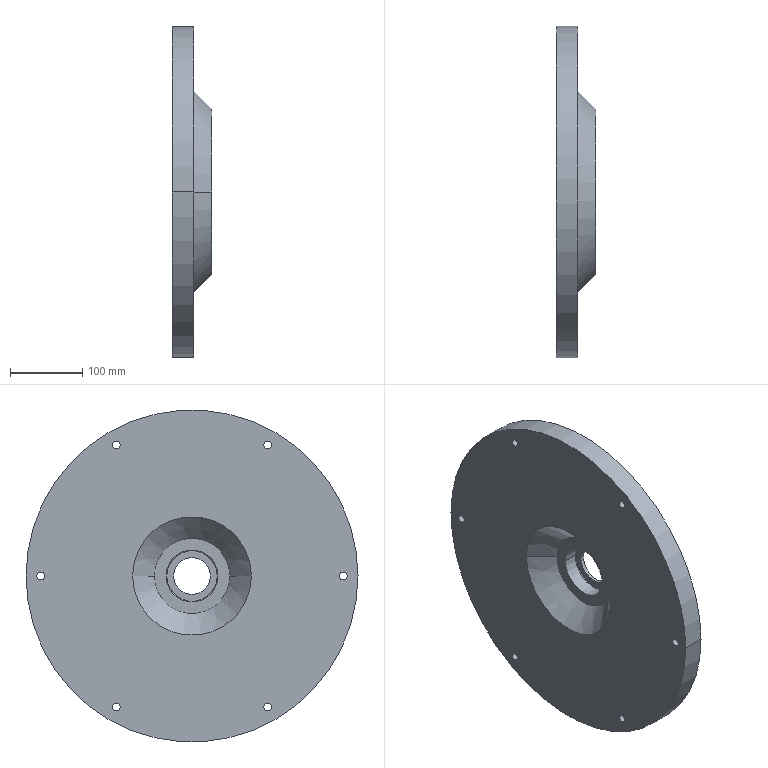Part | SolidWorks | features Cut 1, Revolution 1 | 1 solid | 29 faces | box 55 x 461 x 461 mm | volume 5743075 mm3 | cylinder 18 | plane 5 | cone 4 | torus 2 | commonest cylinder face diameters 11 x12 51 x2 72 x2 461 x2
STEP:
#1=CARTESIAN_POINT('',(-25.,204.5,0.));
#2=VERTEX_POINT('',#1);
#3=CARTESIAN_POINT('',(-25.,215.5,0.));
#4=VERTEX_POINT('',#3);
#5=CARTESIAN_POINT('',(-25.,210.,0.));
#6=DIRECTION('',(1.,0.,0.));
#7=DIRECTION('',(0.,1.,0.));
#8=AXIS2_PLACEMENT_3D('',#5,#6,#7);
#9=CIRCLE('',#8,5.5);
#10=EDGE_CURVE('',#2,#4,#9,.T.);
#11=ORIENTED_EDGE('',*,*,#10,.T.);
#12=CARTESIAN_POINT('',(-55.,215.5,0.));
#13=VERTEX_POINT('',#12);
#14=CARTESIAN_POINT('',(30.,215.5,0.));
#15=DIRECTION('',(-1.,0.,0.));
#16=VECTOR('',#15,1000.);
#17=LINE('',#14,#16);
#18=EDGE_CURVE('',#4,#13,#17,.T.);
#19=ORIENTED_EDGE('',*,*,#18,.T.);
#20=CARTESIAN_POINT('',(-55.,204.5,0.));
#21=VERTEX_POINT('',#20);
#22=CARTESIAN_POINT('',(-55.,210.,0.));
#23=DIRECTION('',(-1.,0.,0.));
#24=DIRECTION('',(0.,-1.,0.));
#25=AXIS2_PLACEMENT_3D('',#22,#23,#24);
#26=CIRCLE('',#25,5.5);
#27=EDGE_CURVE('',#13,#21,#26,.T.);
#28=ORIENTED_EDGE('',*,*,#27,.T.);
#29=CARTESIAN_POINT('',(30.,204.5,0.));
#30=DIRECTION('',(-1.,0.,0.));
#31=VECTOR('',#30,1000.);
#32=LINE('',#29,#31);
#33=EDGE_CURVE('',#2,#21,#32,.T.);
#34=ORIENTED_EDGE('',*,*,#33,.F.);
#35=EDGE_LOOP('',(#11,#19,#28,#34));
#36=FACE_OUTER_BOUND('',#35,.T.);
#37=CARTESIAN_POINT('',(30.,210.,0.));
#38=DIRECTION('',(-1.,0.,0.));
#39=DIRECTION('',(0.,-1.,0.));
#40=AXIS2_PLACEMENT_3D('',#37,#38,#39);
#41=CYLINDRICAL_SURFACE('',#40,5.5);
#42=ADVANCED_FACE('',(#36),#41,.F.);
#43=CARTESIAN_POINT('',(-25.,99.5,-181.865));
#44=VERTEX_POINT('',#43);
#45=CARTESIAN_POINT('',(-25.,110.5,-181.865));
#46=VERTEX_POINT('',#45);
#47=CARTESIAN_POINT('',(-25.,105.,-181.865));
#48=DIRECTION('',(1.,0.,0.));
#49=DIRECTION('',(0.,1.,0.));
#50=AXIS2_PLACEMENT_3D('',#47,#48,#49);
#51=CIRCLE('',#50,5.5);
#52=EDGE_CURVE('',#44,#46,#51,.T.);
#53=ORIENTED_EDGE('',*,*,#52,.T.);
#54=CARTESIAN_POINT('',(-55.,110.5,-181.865));
#55=VERTEX_POINT('',#54);
#56=CARTESIAN_POINT('',(30.,110.5,-181.865));
#57=DIRECTION('',(-1.,0.,0.));
#58=VECTOR('',#57,1000.);
#59=LINE('',#56,#58);
#60=EDGE_CURVE('',#46,#55,#59,.T.);
#61=ORIENTED_EDGE('',*,*,#60,.T.);
#62=CARTESIAN_POINT('',(-55.,99.5,-181.865));
#63=VERTEX_POINT('',#62);
#64=CARTESIAN_POINT('',(-55.,105.,-181.865));
#65=DIRECTION('',(-1.,0.,0.));
#66=DIRECTION('',(0.,-1.,0.));
#67=AXIS2_PLACEMENT_3D('',#64,#65,#66);
#68=CIRCLE('',#67,5.5);
#69=EDGE_CURVE('',#55,#63,#68,.T.);
#70=ORIENTED_EDGE('',*,*,#69,.T.);
#71=CARTESIAN_POINT('',(30.,99.5,-181.865));
#72=DIRECTION('',(-1.,0.,0.));
#73=VECTOR('',#72,1000.);
#74=LINE('',#71,#73);
#75=EDGE_CURVE('',#44,#63,#74,.T.);
#76=ORIENTED_EDGE('',*,*,#75,.F.);
#77=EDGE_LOOP('',(#53,#61,#70,#76));
#78=FACE_OUTER_BOUND('',#77,.T.);
#79=CARTESIAN_POINT('',(30.,105.,-181.865));
#80=DIRECTION('',(-1.,0.,0.));
#81=DIRECTION('',(0.,-1.,0.));
#82=AXIS2_PLACEMENT_3D('',#79,#80,#81);
#83=CYLINDRICAL_SURFACE('',#82,5.5);
#84=ADVANCED_FACE('',(#78),#83,.F.);
#85=CARTESIAN_POINT('',(-25.,-110.5,-181.865));
#86=VERTEX_POINT('',#85);
#87=CARTESIAN_POINT('',(-25.,-99.5,-181.865));
#88=VERTEX_POINT('',#87);
#89=CARTESIAN_POINT('',(-25.,-105.,-181.865));
#90=DIRECTION('',(1.,0.,0.));
#91=DIRECTION('',(0.,1.,0.));
#92=AXIS2_PLACEMENT_3D('',#89,#90,#91);
#93=CIRCLE('',#92,5.5);
#94=EDGE_CURVE('',#86,#88,#93,.T.);
#95=ORIENTED_EDGE('',*,*,#94,.T.);
#96=CARTESIAN_POINT('',(-55.,-99.5,-181.865));
#97=VERTEX_POINT('',#96);
#98=CARTESIAN_POINT('',(30.,-99.5,-181.865));
#99=DIRECTION('',(-1.,0.,0.));
#100=VECTOR('',#99,1000.);
#101=LINE('',#98,#100);
#102=EDGE_CURVE('',#88,#97,#101,.T.);
#103=ORIENTED_EDGE('',*,*,#102,.T.);
#104=CARTESIAN_POINT('',(-55.,-110.5,-181.865));
#105=VERTEX_POINT('',#104);
#106=CARTESIAN_POINT('',(-55.,-105.,-181.865));
#107=DIRECTION('',(-1.,0.,0.));
#108=DIRECTION('',(0.,-1.,0.));
#109=AXIS2_PLACEMENT_3D('',#106,#107,#108);
#110=CIRCLE('',#109,5.5);
#111=EDGE_CURVE('',#97,#105,#110,.T.);
#112=ORIENTED_EDGE('',*,*,#111,.T.);
#113=CARTESIAN_POINT('',(30.,-110.5,-181.865));
#114=DIRECTION('',(-1.,0.,0.));
#115=VECTOR('',#114,1000.);
#116=LINE('',#113,#115);
#117=EDGE_CURVE('',#86,#105,#116,.T.);
#118=ORIENTED_EDGE('',*,*,#117,.F.);
#119=EDGE_LOOP('',(#95,#103,#112,#118));
#120=FACE_OUTER_BOUND('',#119,.T.);
#121=CARTESIAN_POINT('',(30.,-105.,-181.865));
#122=DIRECTION('',(-1.,0.,0.));
#123=DIRECTION('',(0.,-1.,0.));
#124=AXIS2_PLACEMENT_3D('',#121,#122,#123);
#125=CYLINDRICAL_SURFACE('',#124,5.5);
#126=ADVANCED_FACE('',(#120),#125,.F.);
#127=CARTESIAN_POINT('',(-25.,-215.5,0.));
#128=VERTEX_POINT('',#127);
#129=CARTESIAN_POINT('',(-25.,-204.5,0.));
#130=VERTEX_POINT('',#129);
#131=CARTESIAN_POINT('',(-25.,-210.,0.));
#132=DIRECTION('',(1.,0.,0.));
#133=DIRECTION('',(0.,1.,0.));
#134=AXIS2_PLACEMENT_3D('',#131,#132,#133);
#135=CIRCLE('',#134,5.5);
#136=EDGE_CURVE('',#128,#130,#135,.T.);
#137=ORIENTED_EDGE('',*,*,#136,.T.);
#138=CARTESIAN_POINT('',(-55.,-204.5,0.));
#139=VERTEX_POINT('',#138);
#140=CARTESIAN_POINT('',(30.,-204.5,0.));
#141=DIRECTION('',(-1.,0.,0.));
#142=VECTOR('',#141,1000.);
#143=LINE('',#140,#142);
#144=EDGE_CURVE('',#130,#139,#143,.T.);
#145=ORIENTED_EDGE('',*,*,#144,.T.);
#146=CARTESIAN_POINT('',(-55.,-215.5,0.));
#147=VERTEX_POINT('',#146);
#148=CARTESIAN_POINT('',(-55.,-210.,0.));
#149=DIRECTION('',(-1.,0.,0.));
#150=DIRECTION('',(0.,-1.,0.));
#151=AXIS2_PLACEMENT_3D('',#148,#149,#150);
#152=CIRCLE('',#151,5.5);
#153=EDGE_CURVE('',#139,#147,#152,.T.);
#154=ORIENTED_EDGE('',*,*,#153,.T.);
#155=CARTESIAN_POINT('',(30.,-215.5,0.));
#156=DIRECTION('',(-1.,0.,0.));
#157=VECTOR('',#156,1000.);
#158=LINE('',#155,#157);
#159=EDGE_CURVE('',#128,#147,#158,.T.);
#160=ORIENTED_EDGE('',*,*,#159,.F.);
#161=EDGE_LOOP('',(#137,#145,#154,#160));
#162=FACE_OUTER_BOUND('',#161,.T.);
#163=CARTESIAN_POINT('',(30.,-210.,0.));
#164=DIRECTION('',(-1.,0.,0.));
#165=DIRECTION('',(0.,-1.,0.));
#166=AXIS2_PLACEMENT_3D('',#163,#164,#165);
#167=CYLINDRICAL_SURFACE('',#166,5.5);
#168=ADVANCED_FACE('',(#162),#167,.F.);
#169=CARTESIAN_POINT('',(-25.,-110.5,181.865));
#170=VERTEX_POINT('',#169);
#171=CARTESIAN_POINT('',(-25.,-99.5,181.865));
#172=VERTEX_POINT('',#171);
#173=CARTESIAN_POINT('',(-25.,-105.,181.865));
#174=DIRECTION('',(1.,0.,0.));
#175=DIRECTION('',(0.,1.,0.));
#176=AXIS2_PLACEMENT_3D('',#173,#174,#175);
#177=CIRCLE('',#176,5.5);
#178=EDGE_CURVE('',#170,#172,#177,.T.);
#179=ORIENTED_EDGE('',*,*,#178,.T.);
#180=CARTESIAN_POINT('',(-55.,-99.5,181.865));
#181=VERTEX_POINT('',#180);
#182=CARTESIAN_POINT('',(30.,-99.5,181.865));
#183=DIRECTION('',(-1.,0.,0.));
#184=VECTOR('',#183,1000.);
#185=LINE('',#182,#184);
#186=EDGE_CURVE('',#172,#181,#185,.T.);
#187=ORIENTED_EDGE('',*,*,#186,.T.);
#188=CARTESIAN_POINT('',(-55.,-110.5,181.865));
#189=VERTEX_POINT('',#188);
#190=CARTESIAN_POINT('',(-55.,-105.,181.865));
#191=DIRECTION('',(-1.,0.,0.));
#192=DIRECTION('',(0.,-1.,0.));
#193=AXIS2_PLACEMENT_3D('',#190,#191,#192);
#194=CIRCLE('',#193,5.5);
#195=EDGE_CURVE('',#181,#189,#194,.T.);
#196=ORIENTED_EDGE('',*,*,#195,.T.);
#197=CARTESIAN_POINT('',(30.,-110.5,181.865));
#198=DIRECTION('',(-1.,0.,0.));
#199=VECTOR('',#198,1000.);
#200=LINE('',#197,#199);
#201=EDGE_CURVE('',#170,#189,#200,.T.);
#202=ORIENTED_EDGE('',*,*,#201,.F.);
#203=EDGE_LOOP('',(#179,#187,#196,#202));
#204=FACE_OUTER_BOUND('',#203,.T.);
#205=CARTESIAN_POINT('',(30.,-105.,181.865));
#206=DIRECTION('',(-1.,0.,0.));
#207=DIRECTION('',(0.,-1.,0.));
#208=AXIS2_PLACEMENT_3D('',#205,#206,#207);
#209=CYLINDRICAL_SURFACE('',#208,5.5);
#210=ADVANCED_FACE('',(#204),#209,.F.);
#211=CARTESIAN_POINT('',(-25.,99.5,181.865));
#212=VERTEX_POINT('',#211);
#213=CARTESIAN_POINT('',(-25.,110.5,181.865));
#214=VERTEX_POINT('',#213);
#215=CARTESIAN_POINT('',(-25.,105.,181.865));
#216=DIRECTION('',(1.,0.,0.));
#217=DIRECTION('',(0.,1.,0.));
#218=AXIS2_PLACEMENT_3D('',#215,#216,#217);
#219=CIRCLE('',#218,5.5);
#220=EDGE_CURVE('',#212,#214,#219,.T.);
#221=ORIENTED_EDGE('',*,*,#220,.T.);
#222=CARTESIAN_POINT('',(-55.,110.5,181.865));
#223=VERTEX_POINT('',#222);
#224=CARTESIAN_POINT('',(30.,110.5,181.865));
#225=DIRECTION('',(-1.,0.,0.));
#226=VECTOR('',#225,1000.);
#227=LINE('',#224,#226);
#228=EDGE_CURVE('',#214,#223,#227,.T.);
#229=ORIENTED_EDGE('',*,*,#228,.T.);
#230=CARTESIAN_POINT('',(-55.,99.5,181.865));
#231=VERTEX_POINT('',#230);
#232=CARTESIAN_POINT('',(-55.,105.,181.865));
#233=DIRECTION('',(-1.,0.,0.));
#234=DIRECTION('',(0.,-1.,0.));
#235=AXIS2_PLACEMENT_3D('',#232,#233,#234);
#236=CIRCLE('',#235,5.5);
#237=EDGE_CURVE('',#223,#231,#236,.T.);
#238=ORIENTED_EDGE('',*,*,#237,.T.);
#239=CARTESIAN_POINT('',(30.,99.5,181.865));
#240=DIRECTION('',(-1.,0.,0.));
#241=VECTOR('',#240,1000.);
#242=LINE('',#239,#241);
#243=EDGE_CURVE('',#212,#231,#242,.T.);
#244=ORIENTED_EDGE('',*,*,#243,.F.);
#245=EDGE_LOOP('',(#221,#229,#238,#244));
#246=FACE_OUTER_BOUND('',#245,.T.);
#247=CARTESIAN_POINT('',(30.,105.,181.865));
#248=DIRECTION('',(-1.,0.,0.));
#249=DIRECTION('',(0.,-1.,0.));
#250=AXIS2_PLACEMENT_3D('',#247,#248,#249);
#251=CYLINDRICAL_SURFACE('',#250,5.5);
#252=ADVANCED_FACE('',(#246),#251,.F.);
#253=CARTESIAN_POINT('',(0.,115.,0.));
#254=VERTEX_POINT('',#253);
#255=CARTESIAN_POINT('',(0.,-115.,0.));
#256=VERTEX_POINT('',#255);
#257=CARTESIAN_POINT('',(0.,0.,0.));
#258=DIRECTION('',(1.,0.,0.));
#259=DIRECTION('',(0.,1.,0.));
#260=AXIS2_PLACEMENT_3D('',#257,#258,#259);
#261=CIRCLE('',#260,115.);
#262=EDGE_CURVE('',#254,#256,#261,.T.);
#263=ORIENTED_EDGE('',*,*,#262,.F.);
#264=CARTESIAN_POINT('',(-25.,140.,0.));
#265=VERTEX_POINT('',#264);
#266=CARTESIAN_POINT('',(0.,115.,0.));
#267=DIRECTION('',(-0.7071,0.7071,0.));
#268=VECTOR('',#267,1000.);
#269=LINE('',#266,#268);
#270=EDGE_CURVE('',#254,#265,#269,.T.);
#271=ORIENTED_EDGE('',*,*,#270,.T.);
#272=CARTESIAN_POINT('',(-25.,-140.,0.));
#273=VERTEX_POINT('',#272);
#274=CARTESIAN_POINT('',(-25.,0.,0.));
#275=DIRECTION('',(1.,0.,0.));
#276=DIRECTION('',(0.,1.,0.));
#277=AXIS2_PLACEMENT_3D('',#274,#275,#276);
#278=CIRCLE('',#277,140.);
#279=EDGE_CURVE('',#265,#273,#278,.T.);
#280=ORIENTED_EDGE('',*,*,#279,.T.);
#281=CARTESIAN_POINT('',(0.,-115.,0.));
#282=DIRECTION('',(-0.7071,-0.7071,0.));
#283=VECTOR('',#282,1000.);
#284=LINE('',#281,#283);
#285=EDGE_CURVE('',#256,#273,#284,.T.);
#286=ORIENTED_EDGE('',*,*,#285,.F.);
#287=EDGE_LOOP('',(#263,#271,#280,#286));
#288=FACE_OUTER_BOUND('',#287,.T.);
#289=CARTESIAN_POINT('',(0.,0.,0.));
#290=DIRECTION('',(-1.,0.,0.));
#291=DIRECTION('',(0.,-1.,0.));
#292=AXIS2_PLACEMENT_3D('',#289,#290,#291);
#293=CONICAL_SURFACE('',#292,115.,0.7854);
#294=ADVANCED_FACE('',(#288),#293,.T.);
#295=CARTESIAN_POINT('',(-5.,-25.5,0.));
#296=VERTEX_POINT('',#295);
#297=CARTESIAN_POINT('',(-5.,25.5,0.));
#298=VERTEX_POINT('',#297);
#299=CARTESIAN_POINT('',(-5.,0.,0.));
#300=DIRECTION('',(1.,0.,0.));
#301=DIRECTION('',(0.,1.,0.));
#302=AXIS2_PLACEMENT_3D('',#299,#300,#301);
#303=CIRCLE('',#302,25.5);
#304=EDGE_CURVE('',#296,#298,#303,.T.);
#305=ORIENTED_EDGE('',*,*,#304,.F.);
#306=CARTESIAN_POINT('',(0.,-25.5,0.));
#307=VERTEX_POINT('',#306);
#308=CARTESIAN_POINT('',(5.,-25.5,0.));
#309=DIRECTION('',(1.,0.,0.));
#310=VECTOR('',#309,1000.);
#311=LINE('',#308,#310);
#312=EDGE_CURVE('',#296,#307,#311,.T.);
#313=ORIENTED_EDGE('',*,*,#312,.T.);
#314=CARTESIAN_POINT('',(0.,25.5,0.));
#315=VERTEX_POINT('',#314);
#316=CARTESIAN_POINT('',(0.,0.,0.));
#317=DIRECTION('',(1.,0.,0.));
#318=DIRECTION('',(0.,1.,0.));
#319=AXIS2_PLACEMENT_3D('',#316,#317,#318);
#320=CIRCLE('',#319,25.5);
#321=EDGE_CURVE('',#307,#315,#320,.T.);
#322=ORIENTED_EDGE('',*,*,#321,.T.);
#323=CARTESIAN_POINT('',(5.,25.5,0.));
#324=DIRECTION('',(1.,0.,0.));
#325=VECTOR('',#324,1000.);
#326=LINE('',#323,#325);
#327=EDGE_CURVE('',#298,#315,#326,.T.);
#328=ORIENTED_EDGE('',*,*,#327,.F.);
#329=EDGE_LOOP('',(#305,#313,#322,#328));
#330=FACE_OUTER_BOUND('',#329,.T.);
#331=CARTESIAN_POINT('',(5.,0.,0.));
#332=DIRECTION('',(1.,0.,0.));
#333=DIRECTION('',(0.,1.,0.));
#334=AXIS2_PLACEMENT_3D('',#331,#332,#333);
#335=CYLINDRICAL_SURFACE('',#334,25.5);
#336=ADVANCED_FACE('',(#330),#335,.F.);
#337=CARTESIAN_POINT('',(-6.,-36.,0.));
#338=VERTEX_POINT('',#337);
#339=CARTESIAN_POINT('',(-6.,36.,0.));
#340=VERTEX_POINT('',#339);
#341=CARTESIAN_POINT('',(-6.,0.,0.));
#342=DIRECTION('',(1.,0.,0.));
#343=DIRECTION('',(0.,1.,0.));
#344=AXIS2_PLACEMENT_3D('',#341,#342,#343);
#345=CIRCLE('',#344,36.);
#346=EDGE_CURVE('',#338,#340,#345,.T.);
#347=ORIENTED_EDGE('',*,*,#346,.F.);
#348=CARTESIAN_POINT('',(-5.,-35.,0.));
#349=VERTEX_POINT('',#348);
#350=CARTESIAN_POINT('',(-6.,-35.,0.));
#351=DIRECTION('',(0.,0.,1.));
#352=DIRECTION('',(0.,-1.,0.));
#353=AXIS2_PLACEMENT_3D('',#350,#351,#352);
#354=CIRCLE('',#353,1.);
#355=EDGE_CURVE('',#338,#349,#354,.T.);
#356=ORIENTED_EDGE('',*,*,#355,.T.);
#357=CARTESIAN_POINT('',(-5.,35.,0.));
#358=VERTEX_POINT('',#357);
#359=CARTESIAN_POINT('',(-5.,0.,0.));
#360=DIRECTION('',(1.,0.,0.));
#361=DIRECTION('',(0.,1.,0.));
#362=AXIS2_PLACEMENT_3D('',#359,#360,#361);
#363=CIRCLE('',#362,35.);
#364=EDGE_CURVE('',#349,#358,#363,.T.);
#365=ORIENTED_EDGE('',*,*,#364,.T.);
#366=CARTESIAN_POINT('',(-6.,35.,0.));
#367=DIRECTION('',(0.,0.,-1.));
#368=DIRECTION('',(-1.,0.,0.));
#369=AXIS2_PLACEMENT_3D('',#366,#367,#368);
#370=CIRCLE('',#369,1.);
#371=EDGE_CURVE('',#340,#358,#370,.T.);
#372=ORIENTED_EDGE('',*,*,#371,.F.);
#373=EDGE_LOOP('',(#347,#356,#365,#372));
#374=FACE_OUTER_BOUND('',#373,.T.);
#375=CARTESIAN_POINT('',(-6.,0.,0.));
#376=DIRECTION('',(1.,0.,0.));
#377=DIRECTION('',(0.,1.,0.));
#378=AXIS2_PLACEMENT_3D('',#375,#376,#377);
#379=TOROIDAL_SURFACE('',#378,35.,1.);
#380=ADVANCED_FACE('',(#374),#379,.F.);
#381=CARTESIAN_POINT('',(-25.,-36.,0.));
#382=VERTEX_POINT('',#381);
#383=CARTESIAN_POINT('',(-25.,36.,0.));
#384=VERTEX_POINT('',#383);
#385=CARTESIAN_POINT('',(-25.,0.,0.));
#386=DIRECTION('',(1.,0.,0.));
#387=DIRECTION('',(0.,1.,0.));
#388=AXIS2_PLACEMENT_3D('',#385,#386,#387);
#389=CIRCLE('',#388,36.);
#390=EDGE_CURVE('',#382,#384,#389,.T.);
#391=ORIENTED_EDGE('',*,*,#390,.F.);
#392=CARTESIAN_POINT('',(5.,-36.,0.));
#393=DIRECTION('',(1.,0.,0.));
#394=VECTOR('',#393,1000.);
#395=LINE('',#392,#394);
#396=EDGE_CURVE('',#382,#338,#395,.T.);
#397=ORIENTED_EDGE('',*,*,#396,.T.);
#398=ORIENTED_EDGE('',*,*,#346,.T.);
#399=CARTESIAN_POINT('',(5.,36.,0.));
#400=DIRECTION('',(1.,0.,0.));
#401=VECTOR('',#400,1000.);
#402=LINE('',#399,#401);
#403=EDGE_CURVE('',#384,#340,#402,.T.);
#404=ORIENTED_EDGE('',*,*,#403,.F.);
#405=EDGE_LOOP('',(#391,#397,#398,#404));
#406=FACE_OUTER_BOUND('',#405,.T.);
#407=CARTESIAN_POINT('',(5.,0.,0.));
#408=DIRECTION('',(1.,0.,0.));
#409=DIRECTION('',(0.,1.,0.));
#410=AXIS2_PLACEMENT_3D('',#407,#408,#409);
#411=CYLINDRICAL_SURFACE('',#410,36.);
#412=ADVANCED_FACE('',(#406),#411,.F.);
#413=CARTESIAN_POINT('',(-25.,-52.5,0.));
#414=VERTEX_POINT('',#413);
#415=CARTESIAN_POINT('',(-25.,52.5,0.));
#416=VERTEX_POINT('',#415);
#417=CARTESIAN_POINT('',(-25.,0.,0.));
#418=DIRECTION('',(1.,0.,0.));
#419=DIRECTION('',(0.,1.,0.));
#420=AXIS2_PLACEMENT_3D('',#417,#418,#419);
#421=CIRCLE('',#420,52.5);
#422=EDGE_CURVE('',#414,#416,#421,.T.);
#423=ORIENTED_EDGE('',*,*,#422,.T.);
#424=CARTESIAN_POINT('',(-55.,82.5,0.));
#425=VERTEX_POINT('',#424);
#426=CARTESIAN_POINT('',(-55.,82.5,0.));
#427=DIRECTION('',(-0.7071,0.7071,0.));
#428=VECTOR('',#427,1000.);
#429=LINE('',#426,#428);
#430=EDGE_CURVE('',#416,#425,#429,.T.);
#431=ORIENTED_EDGE('',*,*,#430,.T.);
#432=CARTESIAN_POINT('',(-55.,-82.5,0.));
#433=VERTEX_POINT('',#432);
#434=CARTESIAN_POINT('',(-55.,0.,0.));
#435=DIRECTION('',(1.,0.,0.));
#436=DIRECTION('',(0.,1.,0.));
#437=AXIS2_PLACEMENT_3D('',#434,#435,#436);
#438=CIRCLE('',#437,82.5);
#439=EDGE_CURVE('',#433,#425,#438,.T.);
#440=ORIENTED_EDGE('',*,*,#439,.F.);
#441=CARTESIAN_POINT('',(-55.,-82.5,0.));
#442=DIRECTION('',(-0.7071,-0.7071,0.));
#443=VECTOR('',#442,1000.);
#444=LINE('',#441,#443);
#445=EDGE_CURVE('',#414,#433,#444,.T.);
#446=ORIENTED_EDGE('',*,*,#445,.F.);
#447=EDGE_LOOP('',(#423,#431,#440,#446));
#448=FACE_OUTER_BOUND('',#447,.T.);
#449=CARTESIAN_POINT('',(-55.,0.,0.));
#450=DIRECTION('',(-1.,0.,0.));
#451=DIRECTION('',(0.,-1.,0.));
#452=AXIS2_PLACEMENT_3D('',#449,#450,#451);
#453=CONICAL_SURFACE('',#452,82.5,0.7854);
#454=ADVANCED_FACE('',(#448),#453,.F.);
#455=CARTESIAN_POINT('',(-55.,230.5,0.));
#456=VERTEX_POINT('',#455);
#457=CARTESIAN_POINT('',(-55.,-230.5,0.));
#458=VERTEX_POINT('',#457);
#459=CARTESIAN_POINT('',(-55.,0.,0.));
#460=DIRECTION('',(1.,0.,0.));
#461=DIRECTION('',(0.,1.,0.));
#462=AXIS2_PLACEMENT_3D('',#459,#460,#461);
#463=CIRCLE('',#462,230.5);
#464=EDGE_CURVE('',#456,#458,#463,.T.);
#465=ORIENTED_EDGE('',*,*,#464,.T.);
#466=CARTESIAN_POINT('',(-25.,-230.5,0.));
#467=VERTEX_POINT('',#466);
#468=CARTESIAN_POINT('',(5.,-230.5,0.));
#469=DIRECTION('',(1.,0.,0.));
#470=VECTOR('',#469,1000.);
#471=LINE('',#468,#470);
#472=EDGE_CURVE('',#458,#467,#471,.T.);
#473=ORIENTED_EDGE('',*,*,#472,.T.);
#474=CARTESIAN_POINT('',(-25.,230.5,0.));
#475=VERTEX_POINT('',#474);
#476=CARTESIAN_POINT('',(-25.,0.,0.));
#477=DIRECTION('',(1.,0.,0.));
#478=DIRECTION('',(0.,1.,0.));
#479=AXIS2_PLACEMENT_3D('',#476,#477,#478);
#480=CIRCLE('',#479,230.5);
#481=EDGE_CURVE('',#475,#467,#480,.T.);
#482=ORIENTED_EDGE('',*,*,#481,.F.);
#483=CARTESIAN_POINT('',(5.,230.5,0.));
#484=DIRECTION('',(1.,0.,0.));
#485=VECTOR('',#484,1000.);
#486=LINE('',#483,#485);
#487=EDGE_CURVE('',#456,#475,#486,.T.);
#488=ORIENTED_EDGE('',*,*,#487,.F.);
#489=EDGE_LOOP('',(#465,#473,#482,#488));
#490=FACE_OUTER_BOUND('',#489,.T.);
#491=CARTESIAN_POINT('',(5.,0.,0.));
#492=DIRECTION('',(1.,0.,0.));
#493=DIRECTION('',(0.,1.,0.));
#494=AXIS2_PLACEMENT_3D('',#491,#492,#493);
#495=CYLINDRICAL_SURFACE('',#494,230.5);
#496=ADVANCED_FACE('',(#490),#495,.T.);
#497=ORIENTED_EDGE('',*,*,#472,.F.);
#498=CARTESIAN_POINT('',(-55.,0.,0.));
#499=DIRECTION('',(1.,0.,0.));
#500=DIRECTION('',(0.,1.,0.));
#501=AXIS2_PLACEMENT_3D('',#498,#499,#500);
#502=CIRCLE('',#501,230.5);
#503=EDGE_CURVE('',#458,#456,#502,.T.);
#504=ORIENTED_EDGE('',*,*,#503,.T.);
#505=ORIENTED_EDGE('',*,*,#487,.T.);
#506=CARTESIAN_POINT('',(-25.,0.,0.));
#507=DIRECTION('',(1.,0.,0.));
#508=DIRECTION('',(0.,1.,0.));
#509=AXIS2_PLACEMENT_3D('',#506,#507,#508);
#510=CIRCLE('',#509,230.5);
#511=EDGE_CURVE('',#467,#475,#510,.T.);
#512=ORIENTED_EDGE('',*,*,#511,.F.);
#513=EDGE_LOOP('',(#497,#504,#505,#512));
#514=FACE_OUTER_BOUND('',#513,.T.);
#515=CARTESIAN_POINT('',(5.,0.,0.));
#516=DIRECTION('',(1.,0.,0.));
#517=DIRECTION('',(0.,1.,0.));
#518=AXIS2_PLACEMENT_3D('',#515,#516,#517);
#519=CYLINDRICAL_SURFACE('',#518,230.5);
#520=ADVANCED_FACE('',(#514),#519,.T.);
#521=CARTESIAN_POINT('',(-55.,210.,0.));
#522=DIRECTION('',(-1.,0.,0.));
#523=DIRECTION('',(0.,-1.,0.));
#524=AXIS2_PLACEMENT_3D('',#521,#522,#523);
#525=CIRCLE('',#524,5.5);
#526=EDGE_CURVE('',#21,#13,#525,.T.);
#527=ORIENTED_EDGE('',*,*,#526,.F.);
#528=ORIENTED_EDGE('',*,*,#27,.F.);
#529=EDGE_LOOP('',(#527,#528));
#530=FACE_BOUND('',#529,.T.);
#531=CARTESIAN_POINT('',(-55.,105.,-181.865));
#532=DIRECTION('',(-1.,0.,0.));
#533=DIRECTION('',(0.,-1.,0.));
#534=AXIS2_PLACEMENT_3D('',#531,#532,#533);
#535=CIRCLE('',#534,5.5);
#536=EDGE_CURVE('',#63,#55,#535,.T.);
#537=ORIENTED_EDGE('',*,*,#536,.F.);
#538=ORIENTED_EDGE('',*,*,#69,.F.);
#539=EDGE_LOOP('',(#537,#538));
#540=FACE_BOUND('',#539,.T.);
#541=CARTESIAN_POINT('',(-55.,-105.,-181.865));
#542=DIRECTION('',(-1.,0.,0.));
#543=DIRECTION('',(0.,-1.,0.));
#544=AXIS2_PLACEMENT_3D('',#541,#542,#543);
#545=CIRCLE('',#544,5.5);
#546=EDGE_CURVE('',#105,#97,#545,.T.);
#547=ORIENTED_EDGE('',*,*,#546,.F.);
#548=ORIENTED_EDGE('',*,*,#111,.F.);
#549=EDGE_LOOP('',(#547,#548));
#550=FACE_BOUND('',#549,.T.);
#551=CARTESIAN_POINT('',(-55.,-210.,0.));
#552=DIRECTION('',(-1.,0.,0.));
#553=DIRECTION('',(0.,-1.,0.));
#554=AXIS2_PLACEMENT_3D('',#551,#552,#553);
#555=CIRCLE('',#554,5.5);
#556=EDGE_CURVE('',#147,#139,#555,.T.);
#557=ORIENTED_EDGE('',*,*,#556,.F.);
#558=ORIENTED_EDGE('',*,*,#153,.F.);
#559=EDGE_LOOP('',(#557,#558));
#560=FACE_BOUND('',#559,.T.);
#561=CARTESIAN_POINT('',(-55.,-105.,181.865));
#562=DIRECTION('',(-1.,0.,0.));
#563=DIRECTION('',(0.,-1.,0.));
#564=AXIS2_PLACEMENT_3D('',#561,#562,#563);
#565=CIRCLE('',#564,5.5);
#566=EDGE_CURVE('',#189,#181,#565,.T.);
#567=ORIENTED_EDGE('',*,*,#566,.F.);
#568=ORIENTED_EDGE('',*,*,#195,.F.);
#569=EDGE_LOOP('',(#567,#568));
#570=FACE_BOUND('',#569,.T.);
#571=CARTESIAN_POINT('',(-55.,105.,181.865));
#572=DIRECTION('',(-1.,0.,0.));
#573=DIRECTION('',(0.,-1.,0.));
#574=AXIS2_PLACEMENT_3D('',#571,#572,#573);
#575=CIRCLE('',#574,5.5);
#576=EDGE_CURVE('',#231,#223,#575,.T.);
#577=ORIENTED_EDGE('',*,*,#576,.F.);
#578=ORIENTED_EDGE('',*,*,#237,.F.);
#579=EDGE_LOOP('',(#577,#578));
#580=FACE_BOUND('',#579,.T.);
#581=ORIENTED_EDGE('',*,*,#439,.T.);
#582=CARTESIAN_POINT('',(-55.,0.,0.));
#583=DIRECTION('',(1.,0.,0.));
#584=DIRECTION('',(0.,1.,0.));
#585=AXIS2_PLACEMENT_3D('',#582,#583,#584);
#586=CIRCLE('',#585,82.5);
#587=EDGE_CURVE('',#425,#433,#586,.T.);
#588=ORIENTED_EDGE('',*,*,#587,.T.);
#589=EDGE_LOOP('',(#581,#588));
#590=FACE_BOUND('',#589,.T.);
#591=ORIENTED_EDGE('',*,*,#464,.F.);
#592=ORIENTED_EDGE('',*,*,#503,.F.);
#593=EDGE_LOOP('',(#591,#592));
#594=FACE_OUTER_BOUND('',#593,.T.);
#595=CARTESIAN_POINT('',(-55.,205.5,0.));
#596=DIRECTION('',(-1.,0.,0.));
#597=DIRECTION('',(0.,-1.,0.));
#598=AXIS2_PLACEMENT_3D('',#595,#596,#597);
#599=PLANE('',#598);
#600=ADVANCED_FACE('',(#530,#540,#550,#560,#570,#580,#590,#594),#599,.T.);
#601=ORIENTED_EDGE('',*,*,#430,.F.);
#602=CARTESIAN_POINT('',(-25.,0.,0.));
#603=DIRECTION('',(1.,0.,0.));
#604=DIRECTION('',(0.,1.,0.));
#605=AXIS2_PLACEMENT_3D('',#602,#603,#604);
#606=CIRCLE('',#605,52.5);
#607=EDGE_CURVE('',#416,#414,#606,.T.);
#608=ORIENTED_EDGE('',*,*,#607,.T.);
#609=ORIENTED_EDGE('',*,*,#445,.T.);
#610=ORIENTED_EDGE('',*,*,#587,.F.);
#611=EDGE_LOOP('',(#601,#608,#609,#610));
#612=FACE_OUTER_BOUND('',#611,.T.);
#613=CARTESIAN_POINT('',(-55.,0.,0.));
#614=DIRECTION('',(-1.,0.,0.));
#615=DIRECTION('',(0.,-1.,0.));
#616=AXIS2_PLACEMENT_3D('',#613,#614,#615);
#617=CONICAL_SURFACE('',#616,82.5,0.7854);
#618=ADVANCED_FACE('',(#612),#617,.F.);
#619=CARTESIAN_POINT('',(-25.,0.,0.));
#620=DIRECTION('',(1.,0.,0.));
#621=DIRECTION('',(0.,1.,0.));
#622=AXIS2_PLACEMENT_3D('',#619,#620,#621);
#623=CIRCLE('',#622,36.);
#624=EDGE_CURVE('',#384,#382,#623,.T.);
#625=ORIENTED_EDGE('',*,*,#624,.T.);
#626=ORIENTED_EDGE('',*,*,#390,.T.);
#627=EDGE_LOOP('',(#625,#626));
#628=FACE_BOUND('',#627,.T.);
#629=ORIENTED_EDGE('',*,*,#422,.F.);
#630=ORIENTED_EDGE('',*,*,#607,.F.);
#631=EDGE_LOOP('',(#629,#630));
#632=FACE_OUTER_BOUND('',#631,.T.);
#633=CARTESIAN_POINT('',(-25.,36.,0.));
#634=DIRECTION('',(-1.,0.,0.));
#635=DIRECTION('',(0.,-1.,0.));
#636=AXIS2_PLACEMENT_3D('',#633,#634,#635);
#637=PLANE('',#636);
#638=ADVANCED_FACE('',(#628,#632),#637,.T.);
#639=ORIENTED_EDGE('',*,*,#396,.F.);
#640=ORIENTED_EDGE('',*,*,#624,.F.);
#641=ORIENTED_EDGE('',*,*,#403,.T.);
#642=CARTESIAN_POINT('',(-6.,0.,0.));
#643=DIRECTION('',(1.,0.,0.));
#644=DIRECTION('',(0.,1.,0.));
#645=AXIS2_PLACEMENT_3D('',#642,#643,#644);
#646=CIRCLE('',#645,36.);
#647=EDGE_CURVE('',#340,#338,#646,.T.);
#648=ORIENTED_EDGE('',*,*,#647,.T.);
#649=EDGE_LOOP('',(#639,#640,#641,#648));
#650=FACE_OUTER_BOUND('',#649,.T.);
#651=CARTESIAN_POINT('',(5.,0.,0.));
#652=DIRECTION('',(1.,0.,0.));
#653=DIRECTION('',(0.,1.,0.));
#654=AXIS2_PLACEMENT_3D('',#651,#652,#653);
#655=CYLINDRICAL_SURFACE('',#654,36.);
#656=ADVANCED_FACE('',(#650),#655,.F.);
#657=ORIENTED_EDGE('',*,*,#355,.F.);
#658=ORIENTED_EDGE('',*,*,#647,.F.);
#659=ORIENTED_EDGE('',*,*,#371,.T.);
#660=CARTESIAN_POINT('',(-5.,0.,0.));
#661=DIRECTION('',(1.,0.,0.));
#662=DIRECTION('',(0.,1.,0.));
#663=AXIS2_PLACEMENT_3D('',#660,#661,#662);
#664=CIRCLE('',#663,35.);
#665=EDGE_CURVE('',#358,#349,#664,.T.);
#666=ORIENTED_EDGE('',*,*,#665,.T.);
#667=EDGE_LOOP('',(#657,#658,#659,#666));
#668=FACE_OUTER_BOUND('',#667,.T.);
#669=CARTESIAN_POINT('',(-6.,0.,0.));
#670=DIRECTION('',(1.,0.,0.));
#671=DIRECTION('',(0.,1.,0.));
#672=AXIS2_PLACEMENT_3D('',#669,#670,#671);
#673=TOROIDAL_SURFACE('',#672,35.,1.);
#674=ADVANCED_FACE('',(#668),#673,.F.);
#675=CARTESIAN_POINT('',(-5.,0.,0.));
#676=DIRECTION('',(1.,0.,0.));
#677=DIRECTION('',(0.,1.,0.));
#678=AXIS2_PLACEMENT_3D('',#675,#676,#677);
#679=CIRCLE('',#678,25.5);
#680=EDGE_CURVE('',#298,#296,#679,.T.);
#681=ORIENTED_EDGE('',*,*,#680,.T.);
#682=ORIENTED_EDGE('',*,*,#304,.T.);
#683=EDGE_LOOP('',(#681,#682));
#684=FACE_BOUND('',#683,.T.);
#685=ORIENTED_EDGE('',*,*,#665,.F.);
#686=ORIENTED_EDGE('',*,*,#364,.F.);
#687=EDGE_LOOP('',(#685,#686));
#688=FACE_OUTER_BOUND('',#687,.T.);
#689=CARTESIAN_POINT('',(-5.,35.,0.));
#690=DIRECTION('',(-1.,0.,0.));
#691=DIRECTION('',(0.,-1.,0.));
#692=AXIS2_PLACEMENT_3D('',#689,#690,#691);
#693=PLANE('',#692);
#694=ADVANCED_FACE('',(#684,#688),#693,.T.);
#695=ORIENTED_EDGE('',*,*,#312,.F.);
#696=ORIENTED_EDGE('',*,*,#680,.F.);
#697=ORIENTED_EDGE('',*,*,#327,.T.);
#698=CARTESIAN_POINT('',(0.,0.,0.));
#699=DIRECTION('',(1.,0.,0.));
#700=DIRECTION('',(0.,1.,0.));
#701=AXIS2_PLACEMENT_3D('',#698,#699,#700);
#702=CIRCLE('',#701,25.5);
#703=EDGE_CURVE('',#315,#307,#702,.T.);
#704=ORIENTED_EDGE('',*,*,#703,.T.);
#705=EDGE_LOOP('',(#695,#696,#697,#704));
#706=FACE_OUTER_BOUND('',#705,.T.);
#707=CARTESIAN_POINT('',(5.,0.,0.));
#708=DIRECTION('',(1.,0.,0.));
#709=DIRECTION('',(0.,1.,0.));
#710=AXIS2_PLACEMENT_3D('',#707,#708,#709);
#711=CYLINDRICAL_SURFACE('',#710,25.5);
#712=ADVANCED_FACE('',(#706),#711,.F.);
#713=CARTESIAN_POINT('',(0.,0.,0.));
#714=DIRECTION('',(1.,0.,0.));
#715=DIRECTION('',(0.,1.,0.));
#716=AXIS2_PLACEMENT_3D('',#713,#714,#715);
#717=CIRCLE('',#716,115.);
#718=EDGE_CURVE('',#256,#254,#717,.T.);
#719=ORIENTED_EDGE('',*,*,#718,.T.);
#720=ORIENTED_EDGE('',*,*,#262,.T.);
#721=EDGE_LOOP('',(#719,#720));
#722=FACE_OUTER_BOUND('',#721,.T.);
#723=ORIENTED_EDGE('',*,*,#703,.F.);
#724=ORIENTED_EDGE('',*,*,#321,.F.);
#725=EDGE_LOOP('',(#723,#724));
#726=FACE_BOUND('',#725,.T.);
#727=CARTESIAN_POINT('',(0.,115.,0.));
#728=DIRECTION('',(1.,0.,0.));
#729=DIRECTION('',(0.,1.,0.));
#730=AXIS2_PLACEMENT_3D('',#727,#728,#729);
#731=PLANE('',#730);
#732=ADVANCED_FACE('',(#722,#726),#731,.T.);
#733=ORIENTED_EDGE('',*,*,#270,.F.);
#734=ORIENTED_EDGE('',*,*,#718,.F.);
#735=ORIENTED_EDGE('',*,*,#285,.T.);
#736=CARTESIAN_POINT('',(-25.,0.,0.));
#737=DIRECTION('',(1.,0.,0.));
#738=DIRECTION('',(0.,1.,0.));
#739=AXIS2_PLACEMENT_3D('',#736,#737,#738);
#740=CIRCLE('',#739,140.);
#741=EDGE_CURVE('',#273,#265,#740,.T.);
#742=ORIENTED_EDGE('',*,*,#741,.T.);
#743=EDGE_LOOP('',(#733,#734,#735,#742));
#744=FACE_OUTER_BOUND('',#743,.T.);
#745=CARTESIAN_POINT('',(0.,0.,0.));
#746=DIRECTION('',(-1.,0.,0.));
#747=DIRECTION('',(0.,-1.,0.));
#748=AXIS2_PLACEMENT_3D('',#745,#746,#747);
#749=CONICAL_SURFACE('',#748,115.,0.7854);
#750=ADVANCED_FACE('',(#744),#749,.T.);
#751=ORIENTED_EDGE('',*,*,#10,.F.);
#752=CARTESIAN_POINT('',(-25.,210.,0.));
#753=DIRECTION('',(1.,0.,0.));
#754=DIRECTION('',(0.,1.,0.));
#755=AXIS2_PLACEMENT_3D('',#752,#753,#754);
#756=CIRCLE('',#755,5.5);
#757=EDGE_CURVE('',#4,#2,#756,.T.);
#758=ORIENTED_EDGE('',*,*,#757,.F.);
#759=EDGE_LOOP('',(#751,#758));
#760=FACE_BOUND('',#759,.T.);
#761=ORIENTED_EDGE('',*,*,#52,.F.);
#762=CARTESIAN_POINT('',(-25.,105.,-181.865));
#763=DIRECTION('',(1.,0.,0.));
#764=DIRECTION('',(0.,1.,0.));
#765=AXIS2_PLACEMENT_3D('',#762,#763,#764);
#766=CIRCLE('',#765,5.5);
#767=EDGE_CURVE('',#46,#44,#766,.T.);
#768=ORIENTED_EDGE('',*,*,#767,.F.);
#769=EDGE_LOOP('',(#761,#768));
#770=FACE_BOUND('',#769,.T.);
#771=ORIENTED_EDGE('',*,*,#94,.F.);
#772=CARTESIAN_POINT('',(-25.,-105.,-181.865));
#773=DIRECTION('',(1.,0.,0.));
#774=DIRECTION('',(0.,1.,0.));
#775=AXIS2_PLACEMENT_3D('',#772,#773,#774);
#776=CIRCLE('',#775,5.5);
#777=EDGE_CURVE('',#88,#86,#776,.T.);
#778=ORIENTED_EDGE('',*,*,#777,.F.);
#779=EDGE_LOOP('',(#771,#778));
#780=FACE_BOUND('',#779,.T.);
#781=ORIENTED_EDGE('',*,*,#136,.F.);
#782=CARTESIAN_POINT('',(-25.,-210.,0.));
#783=DIRECTION('',(1.,0.,0.));
#784=DIRECTION('',(0.,1.,0.));
#785=AXIS2_PLACEMENT_3D('',#782,#783,#784);
#786=CIRCLE('',#785,5.5);
#787=EDGE_CURVE('',#130,#128,#786,.T.);
#788=ORIENTED_EDGE('',*,*,#787,.F.);
#789=EDGE_LOOP('',(#781,#788));
#790=FACE_BOUND('',#789,.T.);
#791=ORIENTED_EDGE('',*,*,#178,.F.);
#792=CARTESIAN_POINT('',(-25.,-105.,181.865));
#793=DIRECTION('',(1.,0.,0.));
#794=DIRECTION('',(0.,1.,0.));
#795=AXIS2_PLACEMENT_3D('',#792,#793,#794);
#796=CIRCLE('',#795,5.5);
#797=EDGE_CURVE('',#172,#170,#796,.T.);
#798=ORIENTED_EDGE('',*,*,#797,.F.);
#799=EDGE_LOOP('',(#791,#798));
#800=FACE_BOUND('',#799,.T.);
#801=ORIENTED_EDGE('',*,*,#220,.F.);
#802=CARTESIAN_POINT('',(-25.,105.,181.865));
#803=DIRECTION('',(1.,0.,0.));
#804=DIRECTION('',(0.,1.,0.));
#805=AXIS2_PLACEMENT_3D('',#802,#803,#804);
#806=CIRCLE('',#805,5.5);
#807=EDGE_CURVE('',#214,#212,#806,.T.);
#808=ORIENTED_EDGE('',*,*,#807,.F.);
#809=EDGE_LOOP('',(#801,#808));
#810=FACE_BOUND('',#809,.T.);
#811=ORIENTED_EDGE('',*,*,#481,.T.);
#812=ORIENTED_EDGE('',*,*,#511,.T.);
#813=EDGE_LOOP('',(#811,#812));
#814=FACE_OUTER_BOUND('',#813,.T.);
#815=ORIENTED_EDGE('',*,*,#741,.F.);
#816=ORIENTED_EDGE('',*,*,#279,.F.);
#817=EDGE_LOOP('',(#815,#816));
#818=FACE_BOUND('',#817,.T.);
#819=CARTESIAN_POINT('',(-25.,230.5,0.));
#820=DIRECTION('',(1.,0.,0.));
#821=DIRECTION('',(0.,1.,0.));
#822=AXIS2_PLACEMENT_3D('',#819,#820,#821);
#823=PLANE('',#822);
#824=ADVANCED_FACE('',(#760,#770,#780,#790,#800,#810,#814,#818),#823,.T.);
#825=ORIENTED_EDGE('',*,*,#228,.F.);
#826=ORIENTED_EDGE('',*,*,#807,.T.);
#827=ORIENTED_EDGE('',*,*,#243,.T.);
#828=ORIENTED_EDGE('',*,*,#576,.T.);
#829=EDGE_LOOP('',(#825,#826,#827,#828));
#830=FACE_OUTER_BOUND('',#829,.T.);
#831=CARTESIAN_POINT('',(30.,105.,181.865));
#832=DIRECTION('',(-1.,0.,0.));
#833=DIRECTION('',(0.,-1.,0.));
#834=AXIS2_PLACEMENT_3D('',#831,#832,#833);
#835=CYLINDRICAL_SURFACE('',#834,5.5);
#836=ADVANCED_FACE('',(#830),#835,.F.);
#837=ORIENTED_EDGE('',*,*,#186,.F.);
#838=ORIENTED_EDGE('',*,*,#797,.T.);
#839=ORIENTED_EDGE('',*,*,#201,.T.);
#840=ORIENTED_EDGE('',*,*,#566,.T.);
#841=EDGE_LOOP('',(#837,#838,#839,#840));
#842=FACE_OUTER_BOUND('',#841,.T.);
#843=CARTESIAN_POINT('',(30.,-105.,181.865));
#844=DIRECTION('',(-1.,0.,0.));
#845=DIRECTION('',(0.,-1.,0.));
#846=AXIS2_PLACEMENT_3D('',#843,#844,#845);
#847=CYLINDRICAL_SURFACE('',#846,5.5);
#848=ADVANCED_FACE('',(#842),#847,.F.);
#849=ORIENTED_EDGE('',*,*,#144,.F.);
#850=ORIENTED_EDGE('',*,*,#787,.T.);
#851=ORIENTED_EDGE('',*,*,#159,.T.);
#852=ORIENTED_EDGE('',*,*,#556,.T.);
#853=EDGE_LOOP('',(#849,#850,#851,#852));
#854=FACE_OUTER_BOUND('',#853,.T.);
#855=CARTESIAN_POINT('',(30.,-210.,0.));
#856=DIRECTION('',(-1.,0.,0.));
#857=DIRECTION('',(0.,-1.,0.));
#858=AXIS2_PLACEMENT_3D('',#855,#856,#857);
#859=CYLINDRICAL_SURFACE('',#858,5.5);
#860=ADVANCED_FACE('',(#854),#859,.F.);
#861=ORIENTED_EDGE('',*,*,#102,.F.);
#862=ORIENTED_EDGE('',*,*,#777,.T.);
#863=ORIENTED_EDGE('',*,*,#117,.T.);
#864=ORIENTED_EDGE('',*,*,#546,.T.);
#865=EDGE_LOOP('',(#861,#862,#863,#864));
#866=FACE_OUTER_BOUND('',#865,.T.);
#867=CARTESIAN_POINT('',(30.,-105.,-181.865));
#868=DIRECTION('',(-1.,0.,0.));
#869=DIRECTION('',(0.,-1.,0.));
#870=AXIS2_PLACEMENT_3D('',#867,#868,#869);
#871=CYLINDRICAL_SURFACE('',#870,5.5);
#872=ADVANCED_FACE('',(#866),#871,.F.);
#873=ORIENTED_EDGE('',*,*,#60,.F.);
#874=ORIENTED_EDGE('',*,*,#767,.T.);
#875=ORIENTED_EDGE('',*,*,#75,.T.);
#876=ORIENTED_EDGE('',*,*,#536,.T.);
#877=EDGE_LOOP('',(#873,#874,#875,#876));
#878=FACE_OUTER_BOUND('',#877,.T.);
#879=CARTESIAN_POINT('',(30.,105.,-181.865));
#880=DIRECTION('',(-1.,0.,0.));
#881=DIRECTION('',(0.,-1.,0.));
#882=AXIS2_PLACEMENT_3D('',#879,#880,#881);
#883=CYLINDRICAL_SURFACE('',#882,5.5);
#884=ADVANCED_FACE('',(#878),#883,.F.);
#885=ORIENTED_EDGE('',*,*,#18,.F.);
#886=ORIENTED_EDGE('',*,*,#757,.T.);
#887=ORIENTED_EDGE('',*,*,#33,.T.);
#888=ORIENTED_EDGE('',*,*,#526,.T.);
#889=EDGE_LOOP('',(#885,#886,#887,#888));
#890=FACE_OUTER_BOUND('',#889,.T.);
#891=CARTESIAN_POINT('',(30.,210.,0.));
#892=DIRECTION('',(-1.,0.,0.));
#893=DIRECTION('',(0.,-1.,0.));
#894=AXIS2_PLACEMENT_3D('',#891,#892,#893);
#895=CYLINDRICAL_SURFACE('',#894,5.5);
#896=ADVANCED_FACE('',(#890),#895,.F.);
#897=CLOSED_SHELL('',(#42,#84,#126,#168,#210,#252,#294,#336,#380,#412,#454,#496,#520,#600,#618,#638,#656,#674,#694,#712,#732,#750,#824,#836,#848,#860,#872,#884,#896));
#898=MANIFOLD_SOLID_BREP('',#897);
#899=CARTESIAN_POINT('',(0.,0.,0.));
#900=DIRECTION('',(0.,0.,1.));
#901=DIRECTION('',(1.,0.,0.));
#902=AXIS2_PLACEMENT_3D('',#899,#900,#901);
#903=(LENGTH_UNIT()NAMED_UNIT(*)SI_UNIT(.MILLI.,.METRE.));
#904=UNCERTAINTY_MEASURE_WITH_UNIT(LENGTH_MEASURE(0.00001),#903,'','');
#905=(NAMED_UNIT(*)PLANE_ANGLE_UNIT()SI_UNIT($,.RADIAN.));
#906=(NAMED_UNIT(*)SI_UNIT($,.STERADIAN.)SOLID_ANGLE_UNIT());
#907=(GEOMETRIC_REPRESENTATION_CONTEXT(3)GLOBAL_UNCERTAINTY_ASSIGNED_CONTEXT((#904))GLOBAL_UNIT_ASSIGNED_CONTEXT((#903,#905,#906))REPRESENTATION_CONTEXT('',''));
#908=ADVANCED_BREP_SHAPE_REPRESENTATION('',(#898,#902),#907);